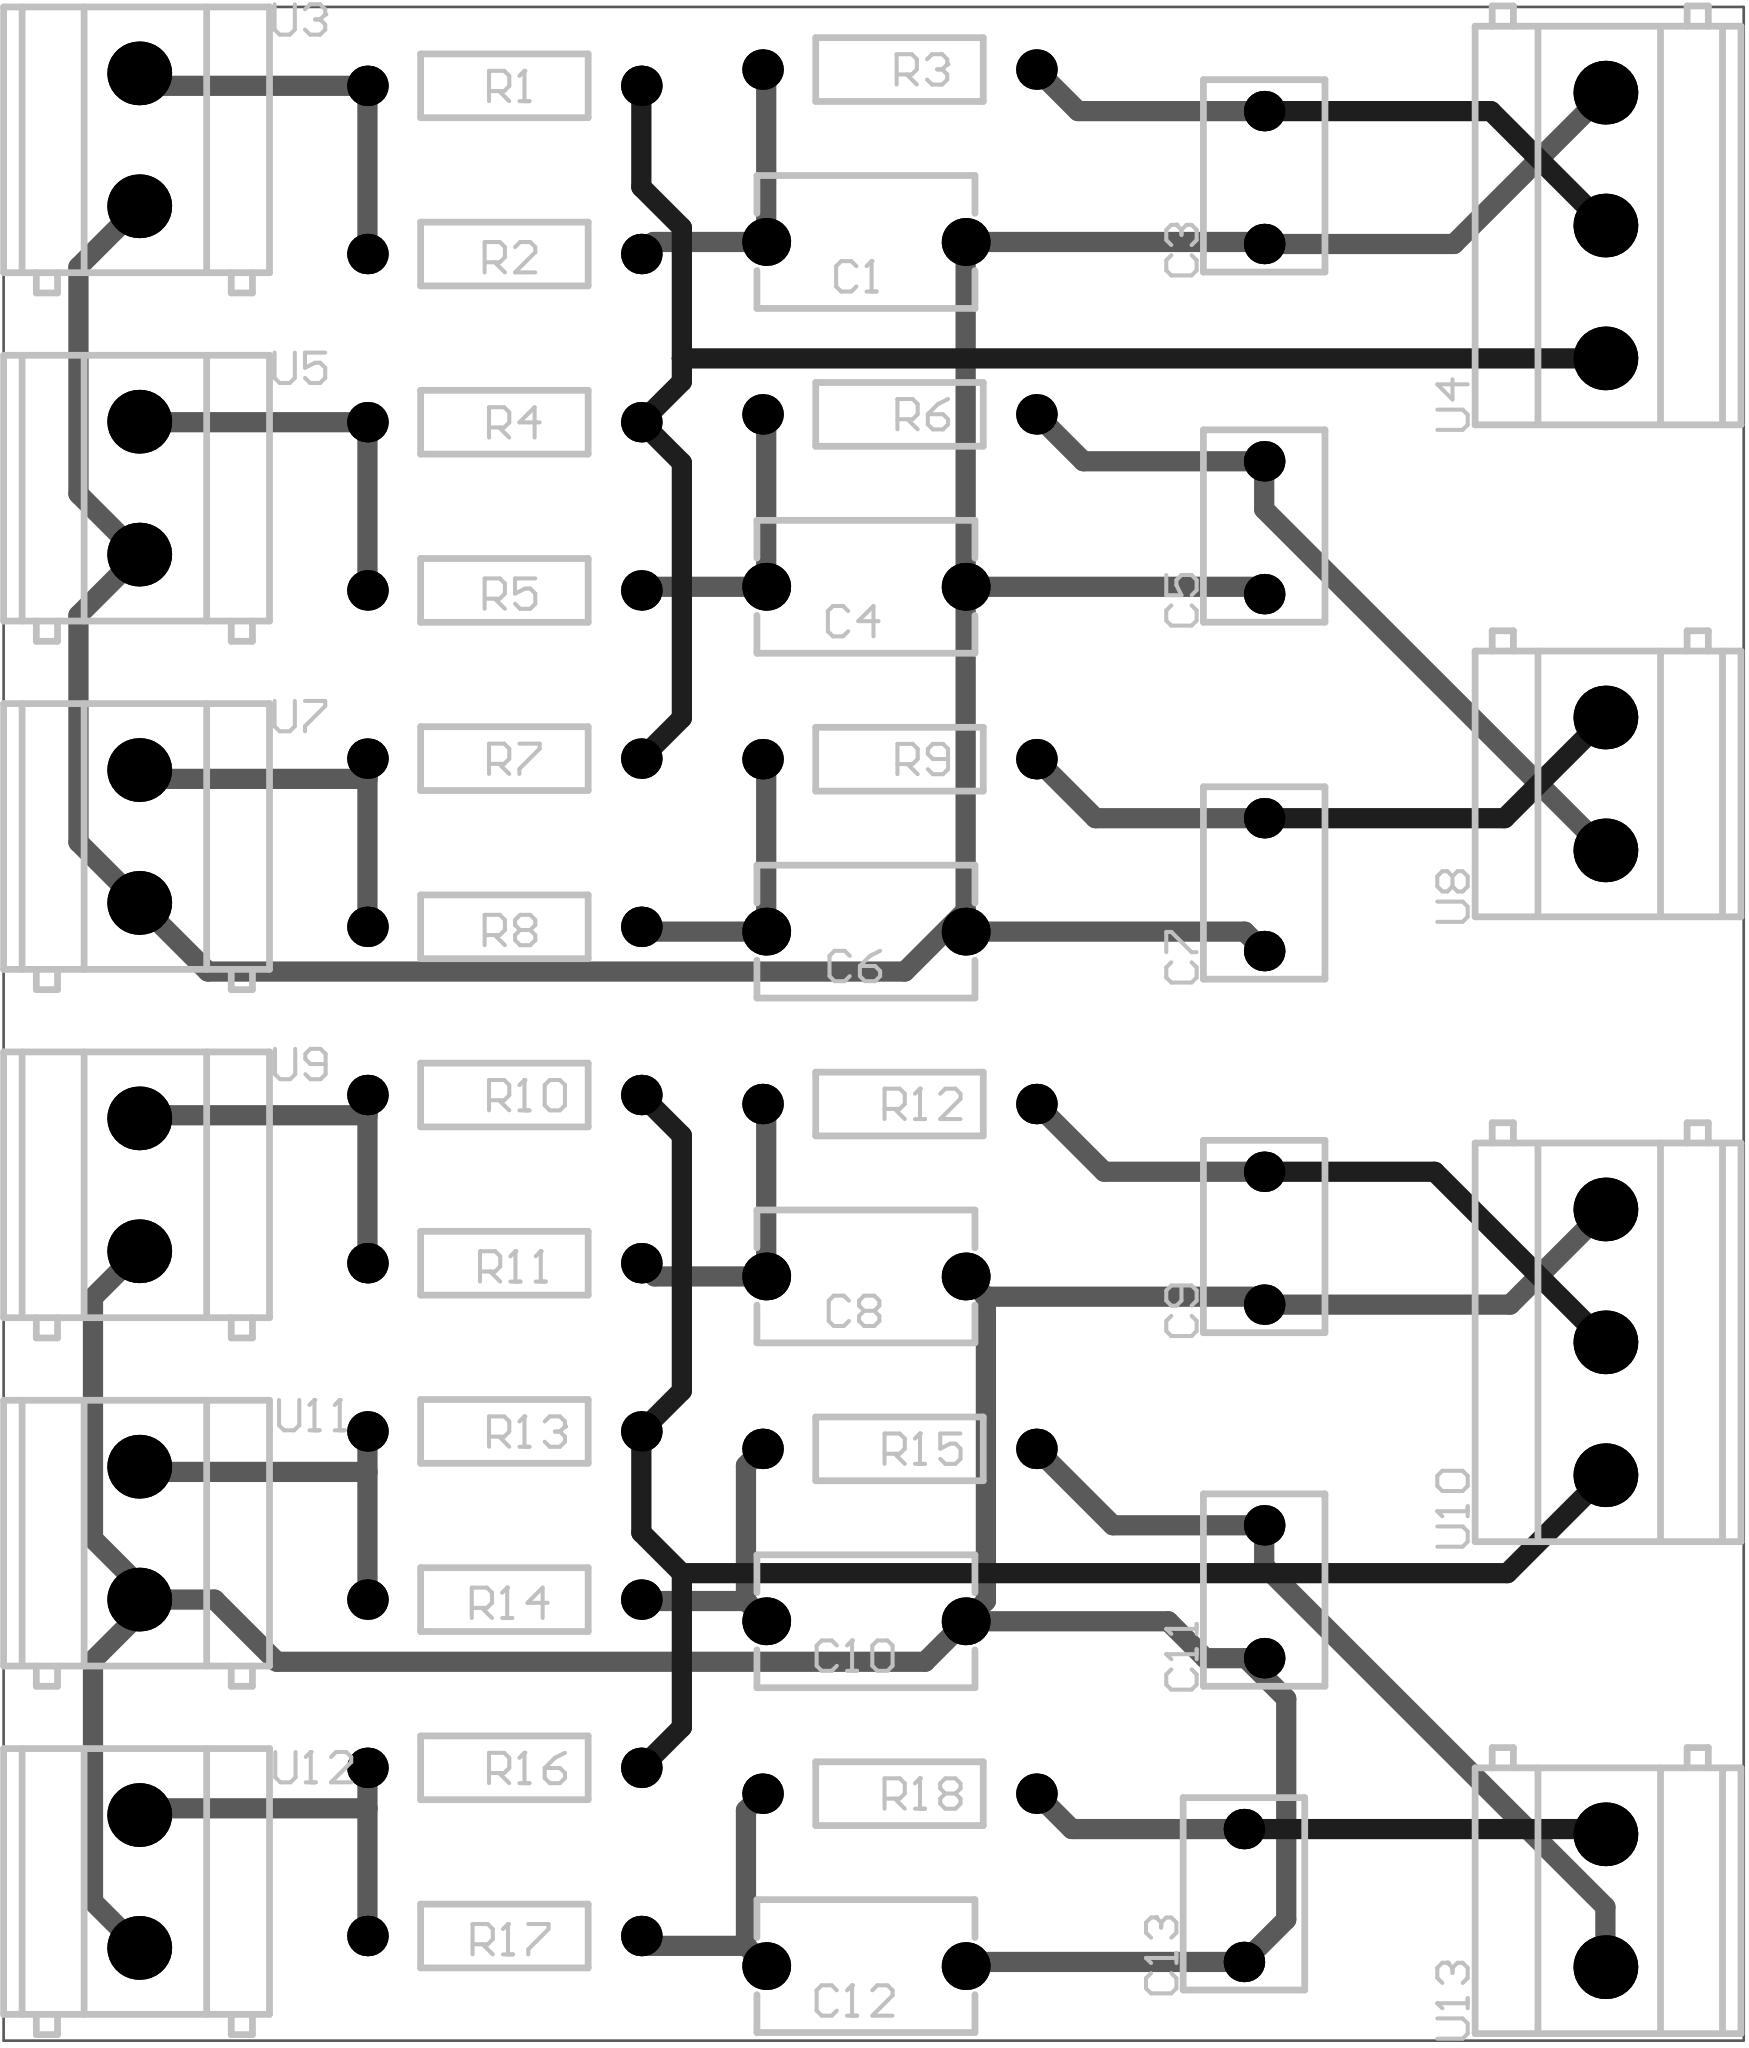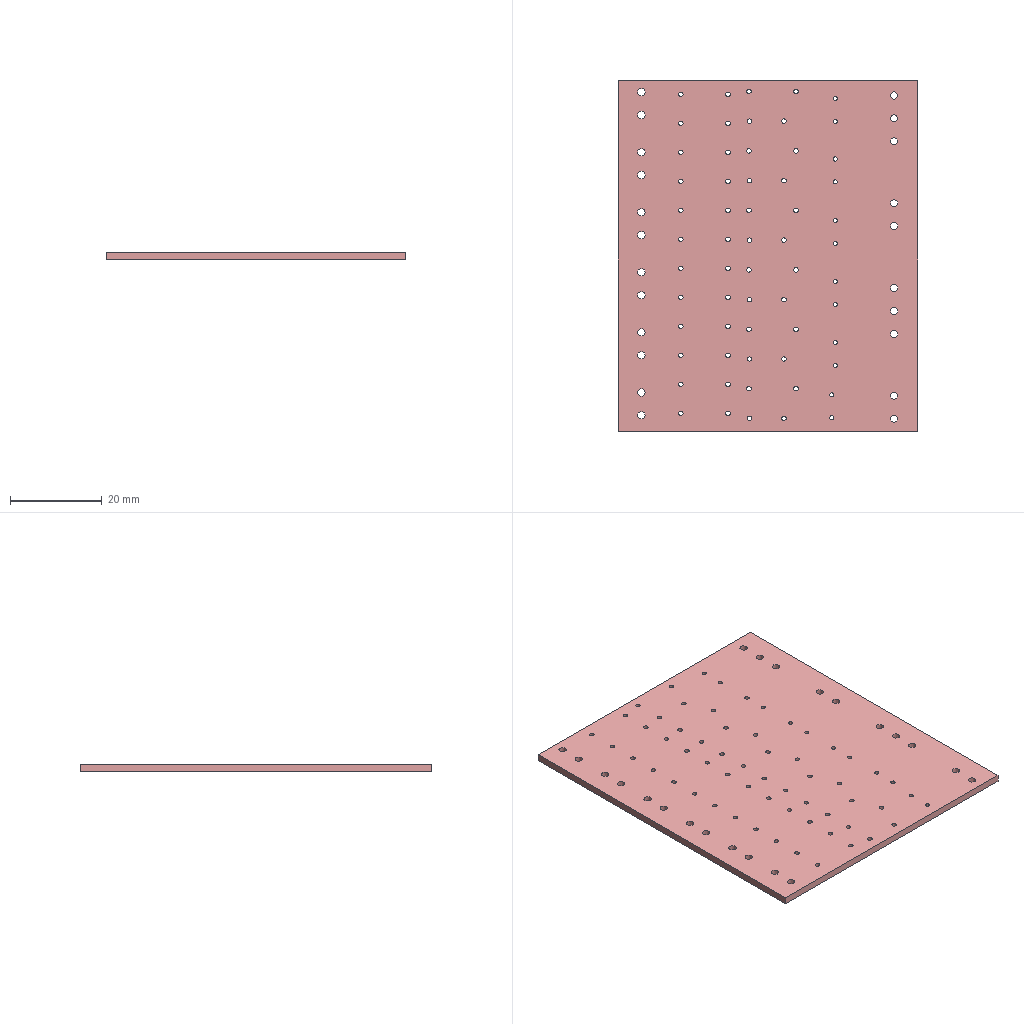Circuit board layout | Altium Designer | box 65.4 x 76.5 x 1.6 mm
Layer stack:
# Altium Designer layer stack of  (unit mm; dielectric type: 0 none, 1 core, 2 prepreg, 3 surface material)
index,name,kind,layer,copper_thickness_mm,dielectric_type,dielectric_thickness_mm,dielectric_material,dielectric_constant
0,Top Paste Mask Layer,other,,,,,,
1,Top Silkscreen Layer,other,,,,,,
2,Top Solder Mask Layer,dielectric,,,3,0.01,,3.3
3,Top Layer,copper,Top Layer,0.035,,,,
4,Dielectric1,dielectric,,,3,1.51,FR4,4.5
5,Bottom Layer,copper,Bottom Layer,0.035,,,,
6,Bottom Solder Mask Layer,dielectric,,,3,0.01,,3.3
7,Bottom Silkscreen Layer,other,,,,,,
8,Bottom Paste Mask Layer,other,,,,,,
# drill layer pairs: low layer,high layer
drill_pair,Top Layer,Bottom Layer
Part placement:
Designator,Comment,Layer,Footprint,Center-X(mm),Center-Y(mm),Rotation
C1,2.2nF,TopLayer,CAP-TH_L8.0-W5.0-P7.50-D1.0,108.817,143.881,180
C3,220pF,TopLayer,CAP-TH_L7.2-W4.5-P5.00-D0.5,123.796,146.304,90
C4,2.2nF,TopLayer,CAP-TH_L8.0-W5.0-P7.50-D1.0,108.817,130.905,180
C5,220pF,TopLayer,CAP-TH_L7.2-W4.5-P5.00-D0.5,123.796,133.128,90
C6,2.2nF,TopLayer,CAP-TH_L8.0-W5.0-P7.50-D1.0,108.817,117.93,180
C7,220pF,TopLayer,CAP-TH_L7.2-W4.5-P5.00-D0.5,123.796,119.698,90
C8,2.2nF,TopLayer,CAP-TH_L8.0-W5.0-P7.50-D1.0,108.817,104.955,180
C9,220pF,TopLayer,CAP-TH_L7.2-W4.5-P5.00-D0.5,123.796,106.394,90
C10,2.2nF,TopLayer,CAP-TH_L8.0-W5.0-P7.50-D1.0,108.817,91.98,180
C11,220pF,TopLayer,CAP-TH_L7.2-W4.5-P5.00-D0.5,123.796,93.091,90
C12,2.2nF,TopLayer,CAP-TH_L8.0-W5.0-P7.50-D1.0,108.817,79.005,180
C13,220pF,TopLayer,CAP-TH_L7.2-W4.5-P5.00-D0.5,123.034,81.661,90
R1,51kΩ,TopLayer,Res_1/4W,95.221,149.756,0
R2,390Ω,TopLayer,Res_1/4W,95.221,143.427,180
R3,3.6kΩ,TopLayer,Res_1/4W,110.08,150.368,180
R4,51kΩ,TopLayer,Res_1/4W,95.221,137.098,0
R5,390Ω,TopLayer,Res_1/4W,95.221,130.769,180
R6,3.6kΩ,TopLayer,Res_1/4W,110.08,137.393,180
R7,51kΩ,TopLayer,Res_1/4W,95.221,124.44,0
R8,390Ω,TopLayer,Res_1/4W,95.221,118.111,180
R9,3.6kΩ,TopLayer,Res_1/4W,110.08,124.418,180
R10,51kΩ,TopLayer,Res_1/4W,95.221,111.782,0
R11,390Ω,TopLayer,Res_1/4W,95.221,105.453,180
R12,3.6kΩ,TopLayer,Res_1/4W,110.08,111.443,180
R13,51kΩ,TopLayer,Res_1/4W,95.221,99.124,0
R14,390Ω,TopLayer,Res_1/4W,95.221,92.795,180
R15,3.6kΩ,TopLayer,Res_1/4W,110.08,98.468,180
R16,51kΩ,TopLayer,Res_1/4W,95.221,86.466,0
R17,390Ω,TopLayer,Res_1/4W,95.221,80.137,180
R18,3.6kΩ,TopLayer,Res_1/4W,110.08,85.493,180
U3,KF128L-5.0-2P,TopLayer,CONN-TH_P5.00_KF128L-5.0-2P,81.487,147.724,270
U4,KF128L-5.0-3P,TopLayer,CONN-TH_3P-P5.00_KF128L-5.0-3P,136.628,144.499,90
U5,KF128L-5.0-2P,TopLayer,CONN-TH_P5.00_KF128L-5.0-2P,81.487,134.617,270
U7,KF128L-5.0-2P,TopLayer,CONN-TH_P5.00_KF128L-5.0-2P,81.487,121.51,270
U8,KF128L-5.0-2P,TopLayer,CONN-TH_P5.00_KF128L-5.0-2P,136.628,123.487,90
U9,KF128L-5.0-2P,TopLayer,CONN-TH_P5.00_KF128L-5.0-2P,81.487,108.403,270
U10,KF128L-5.0-3P,TopLayer,CONN-TH_3P-P5.00_KF128L-5.0-3P,136.628,102.476,90
U11,KF128L-5.0-2P,TopLayer,CONN-TH_P5.00_KF128L-5.0-2P,81.487,95.296,270
U12,KF128L-5.0-2P,TopLayer,CONN-TH_P5.00_KF128L-5.0-2P,81.487,82.189,270
U13,KF128L-5.0-2P,TopLayer,CONN-TH_P5.00_KF128L-5.0-2P,136.628,81.464,90
Pad and via stacks:
# Altium Designer via and pad stacks of  (unit mm). Each distinct definition once, with the count of objects using it.
# via: kind,start_layer,end_layer,hole_mm,diameter_mm,mode(0 simple;1 top-mid-bottom;2 full stack),diameter_per_layer,count,example_net
# pad: kind,layer,hole_mm,hole_type(0 round;1 square;2 slot),plating,top_size,top_shape(1 round;2 rect;3 octagon;9 rounded rect),mid_size,bottom_size,mode,footprint,size_per_layer,count,example
pad,Multi-Layer,1,0,plated,1.8x1.8,1,1.8x1.8,1.8x1.8,0,CAP-TH_L8.0-W5.0-P7.50-D1.0,,12,C1.1
pad,Multi-Layer,0.9144,0,plated,1.524x1.524,1,1.524x1.524,1.524x1.524,0,CAP-TH_L7.2-W4.5-P5.00-D0.5,,12,C3.1
pad,Multi-Layer,1,0,plated,1.524x1.524,1,1.524x1.524,1.524x1.524,0,Res_1/4W,,36,R1.1
pad,Multi-Layer,1.6,0,plated,2.4x2.4,1,2.4x2.4,2.4x2.4,0,CONN-TH_P5.00_KF128L-5.0-2P,,16,U3.1
pad,Multi-Layer,1.6,0,plated,2.4x2.4,1,2.4x2.4,2.4x2.4,0,CONN-TH_3P-P5.00_KF128L-5.0-3P,,6,U4.1
Design rules, without the lines most boards share:
# Altium Designer design rules of  (exported by Altium Designer, unit mm)
# columns: name | kind | enabled | priority | scope1 | scope2 | descriptor | typed fields (field=value)
copperThickness1oz_2 | 2 | enabled | 2 | All | All | Width Constraint (Min=5mil) (Max=100mil) (Preferred=30mil) (All) |
viaSize | 11 | enabled | 1 | All | All | Routing Via (MinHoleWidth=11.811mil) (MaxHoleWidth=248.032mil) (PreferredHoleWidth=12.008mil) (MinWidth=19.685mil) (MaxWidth=393.701mil) (PreferedWidth=24.016mil) (All) | via_min_hole=0.3 via_max_hole=6.3 via_preferred_diameter=0.61 via_preferred_hole=0.305
solderMaskExpansion | 13 | enabled | 2 | All | All | Solder Mask Expansion (Expansion =2.008mil) (All) | expansion=0.051